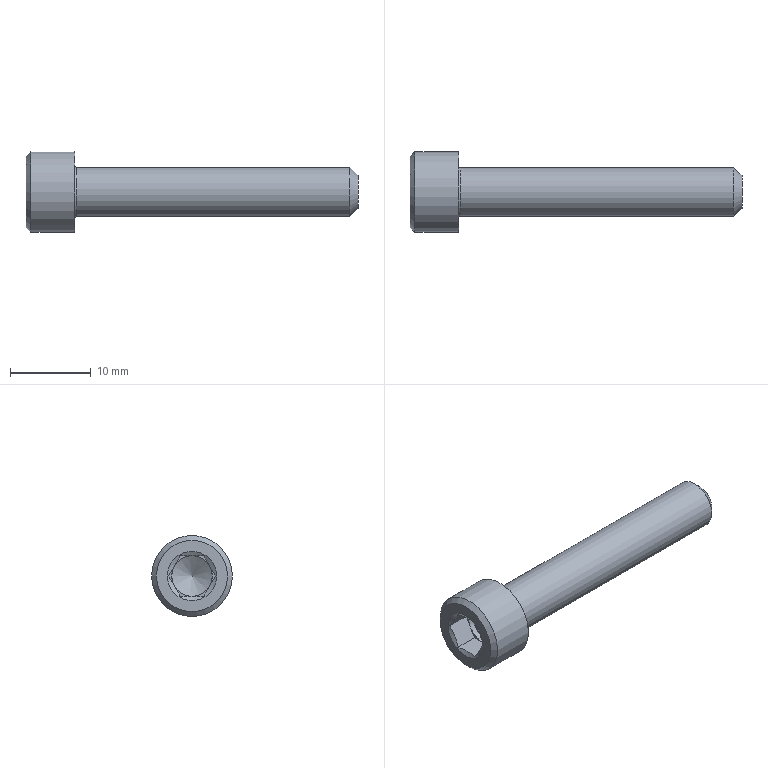Part | STEP file | Винт М6-6gx35 ГОСТ 11738-84 | 1 solid | 23 faces | box 41 x 10 x 10 mm | volume 1358 mm3 | plane 15 | cone 4 | cylinder 3 | torus 1 | commonest cylinder face diameters 5 x1 6 x1 10 x1
STEP:
#1=CARTESIAN_POINT('',(-6.,4.4,0.));
#2=VERTEX_POINT('',#1);
#3=CARTESIAN_POINT('',(-6.,0.,0.));
#4=DIRECTION('',(1.,0.,0.));
#5=DIRECTION('',(0.,1.,0.));
#6=AXIS2_PLACEMENT_3D('',#3,#4,#5);
#7=CIRCLE('',#6,4.4);
#8=EDGE_CURVE('',#2,#2,#7,.T.);
#9=ORIENTED_EDGE('',*,*,#8,.F.);
#10=EDGE_LOOP('',(#9));
#11=FACE_BOUND('',#10,.T.);
#12=CARTESIAN_POINT('',(-6.,3.05,0.));
#13=VERTEX_POINT('',#12);
#14=CARTESIAN_POINT('',(-6.,0.,0.));
#15=DIRECTION('',(1.,0.,0.));
#16=DIRECTION('',(0.,1.,0.));
#17=AXIS2_PLACEMENT_3D('',#14,#15,#16);
#18=CIRCLE('',#17,3.05);
#19=EDGE_CURVE('',#13,#13,#18,.T.);
#20=ORIENTED_EDGE('',*,*,#19,.T.);
#21=EDGE_LOOP('',(#20));
#22=FACE_BOUND('',#21,.T.);
#23=CARTESIAN_POINT('',(-6.,0.,0.));
#24=DIRECTION('',(-1.,0.,0.));
#25=DIRECTION('',(0.,1.,0.));
#26=AXIS2_PLACEMENT_3D('',#23,#24,#25);
#27=PLANE('',#26);
#28=ADVANCED_FACE('',(#11,#22),#27,.T.);
#29=CARTESIAN_POINT('',(-5.906,1.443,-2.5));
#30=VERTEX_POINT('',#29);
#31=CARTESIAN_POINT('',(-5.906,-1.443,-2.5));
#32=VERTEX_POINT('',#31);
#33=CARTESIAN_POINT('',(-5.906,1.443,-2.5));
#34=CARTESIAN_POINT('',(-5.9,1.424,-2.5));
#35=CARTESIAN_POINT('',(-5.89,1.389,-2.5));
#36=CARTESIAN_POINT('',(-5.88,1.351,-2.5));
#37=CARTESIAN_POINT('',(-5.867,1.304,-2.5));
#38=CARTESIAN_POINT('',(-5.848,1.232,-2.5));
#39=CARTESIAN_POINT('',(-5.827,1.146,-2.5));
#40=CARTESIAN_POINT('',(-5.803,1.043,-2.5));
#41=CARTESIAN_POINT('',(-5.774,0.909,-2.5));
#42=CARTESIAN_POINT('',(-5.75,0.7773,-2.5));
#43=CARTESIAN_POINT('',(-5.728,0.6356,-2.5));
#44=CARTESIAN_POINT('',(-5.711,0.5115,-2.5));
#45=CARTESIAN_POINT('',(-5.699,0.3892,-2.5));
#46=CARTESIAN_POINT('',(-5.692,0.2947,-2.5));
#47=CARTESIAN_POINT('',(-5.688,0.2222,-2.5));
#48=CARTESIAN_POINT('',(-5.684,0.1323,-2.5));
#49=CARTESIAN_POINT('',(-5.683,0.05578,-2.5));
#50=CARTESIAN_POINT('',(-5.682,-0.001577,-2.5));
#51=CARTESIAN_POINT('',(-5.683,-0.03169,-2.5));
#52=CARTESIAN_POINT('',(-5.683,-0.0738,-2.5));
#53=CARTESIAN_POINT('',(-5.684,-0.1276,-2.5));
#54=CARTESIAN_POINT('',(-5.687,-0.2055,-2.5));
#55=CARTESIAN_POINT('',(-5.692,-0.2839,-2.5));
#56=CARTESIAN_POINT('',(-5.696,-0.3444,-2.5));
#57=CARTESIAN_POINT('',(-5.7,-0.3959,-2.5));
#58=CARTESIAN_POINT('',(-5.705,-0.4472,-2.5));
#59=CARTESIAN_POINT('',(-5.713,-0.5148,-2.5));
#60=CARTESIAN_POINT('',(-5.722,-0.5907,-2.5));
#61=CARTESIAN_POINT('',(-5.73,-0.6507,-2.5));
#62=CARTESIAN_POINT('',(-5.738,-0.7005,-2.5));
#63=CARTESIAN_POINT('',(-5.746,-0.7498,-2.5));
#64=CARTESIAN_POINT('',(-5.757,-0.8136,-2.5));
#65=CARTESIAN_POINT('',(-5.77,-0.8864,-2.5));
#66=CARTESIAN_POINT('',(-5.785,-0.9583,-2.5));
#67=CARTESIAN_POINT('',(-5.8,-1.03,-2.5));
#68=CARTESIAN_POINT('',(-5.812,-1.084,-2.5));
#69=CARTESIAN_POINT('',(-5.823,-1.131,-2.5));
#70=CARTESIAN_POINT('',(-5.834,-1.177,-2.5));
#71=CARTESIAN_POINT('',(-5.85,-1.239,-2.5));
#72=CARTESIAN_POINT('',(-5.868,-1.307,-2.5));
#73=CARTESIAN_POINT('',(-5.882,-1.361,-2.5));
#74=CARTESIAN_POINT('',(-5.895,-1.406,-2.5));
#75=CARTESIAN_POINT('',(-5.902,-1.429,-2.5));
#76=CARTESIAN_POINT('',(-5.906,-1.443,-2.5));
#77=B_SPLINE_CURVE_WITH_KNOTS('',3,(#33,#34,#35,#36,#37,#38,#39,#40,#41,#42,#43,#44,#45,#46,#47,#48,#49,#50,#51,#52,#53,#54,#55,#56,#57,#58,#59,#60,#61,#62,#63,#64,#65,#66,#67,#68,#69,#70,#71,#72,#73,#74,#75,#76),.UNSPECIFIED.,.F.,.F.,(4,1,1,1,1,1,1,1,1,1,1,1,1,1,1,1,1,1,1,1,1,1,1,1,1,1,1,1,1,1,1,1,1,1,1,1,1,1,1,1,1,4),(0.,0.02097,0.03685,0.04095,0.07015,0.1134,0.1316,0.1778,0.2541,0.2686,0.3246,0.3823,0.3943,0.4217,0.4566,0.4863,0.5,0.5153,0.5171,0.5431,0.5703,0.5969,0.6234,0.6325,0.6498,0.6761,0.7022,0.7281,0.7381,0.7538,0.7792,0.8044,0.8294,0.8543,0.8789,0.8866,0.9033,0.9276,0.9518,0.9759,0.9843,1.),.UNSPECIFIED.);
#78=EDGE_CURVE('',#30,#32,#77,.T.);
#79=ORIENTED_EDGE('',*,*,#78,.T.);
#80=CARTESIAN_POINT('',(-3.,-1.443,-2.5));
#81=VERTEX_POINT('',#80);
#82=CARTESIAN_POINT('',(-3.,-1.443,-2.5));
#83=DIRECTION('',(-1.,0.,0.));
#84=VECTOR('',#83,1.);
#85=LINE('',#82,#84);
#86=EDGE_CURVE('',#81,#32,#85,.T.);
#87=ORIENTED_EDGE('',*,*,#86,.F.);
#88=CARTESIAN_POINT('',(-3.,0.,-2.5));
#89=VERTEX_POINT('',#88);
#90=CARTESIAN_POINT('',(-3.,0.,-2.5));
#91=DIRECTION('',(0.,-1.,0.));
#92=VECTOR('',#91,1.);
#93=LINE('',#90,#92);
#94=EDGE_CURVE('',#89,#81,#93,.T.);
#95=ORIENTED_EDGE('',*,*,#94,.F.);
#96=CARTESIAN_POINT('',(-3.,1.443,-2.5));
#97=VERTEX_POINT('',#96);
#98=CARTESIAN_POINT('',(-3.,1.443,-2.5));
#99=DIRECTION('',(0.,-1.,0.));
#100=VECTOR('',#99,1.);
#101=LINE('',#98,#100);
#102=EDGE_CURVE('',#97,#89,#101,.T.);
#103=ORIENTED_EDGE('',*,*,#102,.F.);
#104=CARTESIAN_POINT('',(-3.,1.443,-2.5));
#105=DIRECTION('',(-1.,0.,0.));
#106=VECTOR('',#105,1.);
#107=LINE('',#104,#106);
#108=EDGE_CURVE('',#97,#30,#107,.T.);
#109=ORIENTED_EDGE('',*,*,#108,.T.);
#110=EDGE_LOOP('',(#79,#87,#95,#103,#109));
#111=FACE_BOUND('',#110,.T.);
#112=CARTESIAN_POINT('',(-3.,1.443,-2.5));
#113=DIRECTION('',(0.,0.,-1.));
#114=DIRECTION('',(0.,-1.,0.));
#115=AXIS2_PLACEMENT_3D('',#112,#113,#114);
#116=PLANE('',#115);
#117=ADVANCED_FACE('',(#111),#116,.F.);
#118=CARTESIAN_POINT('',(-5.906,-2.887,0.));
#119=VERTEX_POINT('',#118);
#120=CARTESIAN_POINT('',(-5.906,-1.443,-2.5));
#121=CARTESIAN_POINT('',(-5.9,-1.453,-2.483));
#122=CARTESIAN_POINT('',(-5.889,-1.472,-2.45));
#123=CARTESIAN_POINT('',(-5.871,-1.505,-2.392));
#124=CARTESIAN_POINT('',(-5.848,-1.549,-2.317));
#125=CARTESIAN_POINT('',(-5.816,-1.614,-2.204));
#126=CARTESIAN_POINT('',(-5.777,-1.702,-2.052));
#127=CARTESIAN_POINT('',(-5.74,-1.803,-1.877));
#128=CARTESIAN_POINT('',(-5.713,-1.902,-1.705));
#129=CARTESIAN_POINT('',(-5.697,-1.984,-1.564));
#130=CARTESIAN_POINT('',(-5.688,-2.048,-1.453));
#131=CARTESIAN_POINT('',(-5.684,-2.099,-1.365));
#132=CARTESIAN_POINT('',(-5.683,-2.137,-1.298));
#133=CARTESIAN_POINT('',(-5.682,-2.166,-1.249));
#134=CARTESIAN_POINT('',(-5.683,-2.194,-1.201));
#135=CARTESIAN_POINT('',(-5.684,-2.228,-1.141));
#136=CARTESIAN_POINT('',(-5.687,-2.268,-1.072));
#137=CARTESIAN_POINT('',(-5.692,-2.307,-1.004));
#138=CARTESIAN_POINT('',(-5.697,-2.346,-0.9371));
#139=CARTESIAN_POINT('',(-5.704,-2.384,-0.8704));
#140=CARTESIAN_POINT('',(-5.713,-2.422,-0.8041));
#141=CARTESIAN_POINT('',(-5.722,-2.46,-0.7384));
#142=CARTESIAN_POINT('',(-5.733,-2.498,-0.6734));
#143=CARTESIAN_POINT('',(-5.744,-2.535,-0.609));
#144=CARTESIAN_POINT('',(-5.757,-2.572,-0.5454));
#145=CARTESIAN_POINT('',(-5.77,-2.608,-0.4824));
#146=CARTESIAN_POINT('',(-5.785,-2.644,-0.4201));
#147=CARTESIAN_POINT('',(-5.8,-2.68,-0.3584));
#148=CARTESIAN_POINT('',(-5.816,-2.715,-0.2974));
#149=CARTESIAN_POINT('',(-5.832,-2.75,-0.237));
#150=CARTESIAN_POINT('',(-5.85,-2.784,-0.1771));
#151=CARTESIAN_POINT('',(-5.868,-2.819,-0.1177));
#152=CARTESIAN_POINT('',(-5.886,-2.853,-0.05869));
#153=CARTESIAN_POINT('',(-5.899,-2.875,-0.01952));
#154=CARTESIAN_POINT('',(-5.906,-2.887,0.));
#155=B_SPLINE_CURVE_WITH_KNOTS('',3,(#120,#121,#122,#123,#124,#125,#126,#127,#128,#129,#130,#131,#132,#133,#134,#135,#136,#137,#138,#139,#140,#141,#142,#143,#144,#145,#146,#147,#148,#149,#150,#151,#152,#153,#154),.UNSPECIFIED.,.F.,.F.,(4,1,1,1,1,1,1,1,1,1,1,1,1,1,1,1,1,1,1,1,1,1,1,1,1,1,1,1,1,1,1,1,4),(0.,0.02097,0.04095,0.07015,0.1134,0.1778,0.2541,0.3246,0.3823,0.4217,0.4566,0.4863,0.5,0.5153,0.5431,0.5703,0.5969,0.6234,0.6498,0.6761,0.7022,0.7281,0.7538,0.7792,0.8044,0.8294,0.8543,0.8789,0.9033,0.9276,0.9518,0.9759,1.),.UNSPECIFIED.);
#156=EDGE_CURVE('',#32,#119,#155,.T.);
#157=ORIENTED_EDGE('',*,*,#156,.T.);
#158=CARTESIAN_POINT('',(-3.,-2.887,0.));
#159=VERTEX_POINT('',#158);
#160=CARTESIAN_POINT('',(-3.,-2.887,0.));
#161=DIRECTION('',(-1.,0.,0.));
#162=VECTOR('',#161,1.);
#163=LINE('',#160,#162);
#164=EDGE_CURVE('',#159,#119,#163,.T.);
#165=ORIENTED_EDGE('',*,*,#164,.F.);
#166=CARTESIAN_POINT('',(-3.,-2.165,-1.25));
#167=VERTEX_POINT('',#166);
#168=CARTESIAN_POINT('',(-3.,-2.165,-1.25));
#169=DIRECTION('',(0.,-0.5,0.866));
#170=VECTOR('',#169,1.);
#171=LINE('',#168,#170);
#172=EDGE_CURVE('',#167,#159,#171,.T.);
#173=ORIENTED_EDGE('',*,*,#172,.F.);
#174=CARTESIAN_POINT('',(-3.,-1.443,-2.5));
#175=DIRECTION('',(0.,-0.5,0.866));
#176=VECTOR('',#175,1.);
#177=LINE('',#174,#176);
#178=EDGE_CURVE('',#81,#167,#177,.T.);
#179=ORIENTED_EDGE('',*,*,#178,.F.);
#180=ORIENTED_EDGE('',*,*,#86,.T.);
#181=EDGE_LOOP('',(#157,#165,#173,#179,#180));
#182=FACE_BOUND('',#181,.T.);
#183=CARTESIAN_POINT('',(-3.,-1.443,-2.5));
#184=DIRECTION('',(0.,-0.866,-0.5));
#185=DIRECTION('',(0.,-0.5,0.866));
#186=AXIS2_PLACEMENT_3D('',#183,#184,#185);
#187=PLANE('',#186);
#188=ADVANCED_FACE('',(#182),#187,.F.);
#189=CARTESIAN_POINT('',(-5.906,-1.443,2.5));
#190=VERTEX_POINT('',#189);
#191=CARTESIAN_POINT('',(-5.906,-2.887,0.));
#192=CARTESIAN_POINT('',(-5.9,-2.877,0.01704));
#193=CARTESIAN_POINT('',(-5.889,-2.858,0.05036));
#194=CARTESIAN_POINT('',(-5.871,-2.825,0.1076));
#195=CARTESIAN_POINT('',(-5.848,-2.781,0.1832));
#196=CARTESIAN_POINT('',(-5.816,-2.716,0.2956));
#197=CARTESIAN_POINT('',(-5.777,-2.628,0.4476));
#198=CARTESIAN_POINT('',(-5.74,-2.527,0.6235));
#199=CARTESIAN_POINT('',(-5.713,-2.428,0.7948));
#200=CARTESIAN_POINT('',(-5.697,-2.346,0.936));
#201=CARTESIAN_POINT('',(-5.688,-2.282,1.047));
#202=CARTESIAN_POINT('',(-5.684,-2.231,1.135));
#203=CARTESIAN_POINT('',(-5.683,-2.193,1.202));
#204=CARTESIAN_POINT('',(-5.682,-2.164,1.251));
#205=CARTESIAN_POINT('',(-5.683,-2.137,1.299));
#206=CARTESIAN_POINT('',(-5.684,-2.102,1.359));
#207=CARTESIAN_POINT('',(-5.687,-2.062,1.428));
#208=CARTESIAN_POINT('',(-5.692,-2.023,1.496));
#209=CARTESIAN_POINT('',(-5.697,-1.984,1.563));
#210=CARTESIAN_POINT('',(-5.704,-1.946,1.63));
#211=CARTESIAN_POINT('',(-5.713,-1.908,1.696));
#212=CARTESIAN_POINT('',(-5.722,-1.87,1.762));
#213=CARTESIAN_POINT('',(-5.733,-1.832,1.827));
#214=CARTESIAN_POINT('',(-5.744,-1.795,1.891));
#215=CARTESIAN_POINT('',(-5.757,-1.758,1.955));
#216=CARTESIAN_POINT('',(-5.77,-1.722,2.018));
#217=CARTESIAN_POINT('',(-5.785,-1.686,2.08));
#218=CARTESIAN_POINT('',(-5.8,-1.65,2.142));
#219=CARTESIAN_POINT('',(-5.816,-1.615,2.203));
#220=CARTESIAN_POINT('',(-5.832,-1.58,2.263));
#221=CARTESIAN_POINT('',(-5.85,-1.546,2.323));
#222=CARTESIAN_POINT('',(-5.868,-1.511,2.382));
#223=CARTESIAN_POINT('',(-5.886,-1.477,2.441));
#224=CARTESIAN_POINT('',(-5.899,-1.455,2.48));
#225=CARTESIAN_POINT('',(-5.906,-1.443,2.5));
#226=B_SPLINE_CURVE_WITH_KNOTS('',3,(#191,#192,#193,#194,#195,#196,#197,#198,#199,#200,#201,#202,#203,#204,#205,#206,#207,#208,#209,#210,#211,#212,#213,#214,#215,#216,#217,#218,#219,#220,#221,#222,#223,#224,#225),.UNSPECIFIED.,.F.,.F.,(4,1,1,1,1,1,1,1,1,1,1,1,1,1,1,1,1,1,1,1,1,1,1,1,1,1,1,1,1,1,1,1,4),(0.,0.02097,0.04095,0.07015,0.1134,0.1778,0.2541,0.3246,0.3823,0.4217,0.4566,0.4863,0.5,0.5153,0.5431,0.5703,0.5969,0.6234,0.6498,0.6761,0.7022,0.7281,0.7538,0.7792,0.8044,0.8294,0.8543,0.8789,0.9033,0.9276,0.9518,0.9759,1.),.UNSPECIFIED.);
#227=EDGE_CURVE('',#119,#190,#226,.T.);
#228=ORIENTED_EDGE('',*,*,#227,.T.);
#229=CARTESIAN_POINT('',(-3.,-1.443,2.5));
#230=VERTEX_POINT('',#229);
#231=CARTESIAN_POINT('',(-3.,-1.443,2.5));
#232=DIRECTION('',(-1.,0.,0.));
#233=VECTOR('',#232,1.);
#234=LINE('',#231,#233);
#235=EDGE_CURVE('',#230,#190,#234,.T.);
#236=ORIENTED_EDGE('',*,*,#235,.F.);
#237=CARTESIAN_POINT('',(-3.,-2.165,1.25));
#238=VERTEX_POINT('',#237);
#239=CARTESIAN_POINT('',(-3.,-2.165,1.25));
#240=DIRECTION('',(0.,0.5,0.866));
#241=VECTOR('',#240,1.);
#242=LINE('',#239,#241);
#243=EDGE_CURVE('',#238,#230,#242,.T.);
#244=ORIENTED_EDGE('',*,*,#243,.F.);
#245=CARTESIAN_POINT('',(-3.,-2.887,0.));
#246=DIRECTION('',(0.,0.5,0.866));
#247=VECTOR('',#246,1.);
#248=LINE('',#245,#247);
#249=EDGE_CURVE('',#159,#238,#248,.T.);
#250=ORIENTED_EDGE('',*,*,#249,.F.);
#251=ORIENTED_EDGE('',*,*,#164,.T.);
#252=EDGE_LOOP('',(#228,#236,#244,#250,#251));
#253=FACE_BOUND('',#252,.T.);
#254=CARTESIAN_POINT('',(-3.,-2.887,0.));
#255=DIRECTION('',(0.,-0.866,0.5));
#256=DIRECTION('',(0.,0.5,0.866));
#257=AXIS2_PLACEMENT_3D('',#254,#255,#256);
#258=PLANE('',#257);
#259=ADVANCED_FACE('',(#253),#258,.F.);
#260=CARTESIAN_POINT('',(-5.906,1.443,2.5));
#261=VERTEX_POINT('',#260);
#262=CARTESIAN_POINT('',(-5.906,-1.443,2.5));
#263=CARTESIAN_POINT('',(-5.9,-1.424,2.5));
#264=CARTESIAN_POINT('',(-5.89,-1.389,2.5));
#265=CARTESIAN_POINT('',(-5.88,-1.351,2.5));
#266=CARTESIAN_POINT('',(-5.867,-1.304,2.5));
#267=CARTESIAN_POINT('',(-5.848,-1.232,2.5));
#268=CARTESIAN_POINT('',(-5.827,-1.146,2.5));
#269=CARTESIAN_POINT('',(-5.803,-1.043,2.5));
#270=CARTESIAN_POINT('',(-5.774,-0.909,2.5));
#271=CARTESIAN_POINT('',(-5.75,-0.7773,2.5));
#272=CARTESIAN_POINT('',(-5.728,-0.6356,2.5));
#273=CARTESIAN_POINT('',(-5.711,-0.5115,2.5));
#274=CARTESIAN_POINT('',(-5.699,-0.3892,2.5));
#275=CARTESIAN_POINT('',(-5.692,-0.2947,2.5));
#276=CARTESIAN_POINT('',(-5.688,-0.2222,2.5));
#277=CARTESIAN_POINT('',(-5.684,-0.1323,2.5));
#278=CARTESIAN_POINT('',(-5.683,-0.05578,2.5));
#279=CARTESIAN_POINT('',(-5.682,0.001577,2.5));
#280=CARTESIAN_POINT('',(-5.683,0.03169,2.5));
#281=CARTESIAN_POINT('',(-5.683,0.0738,2.5));
#282=CARTESIAN_POINT('',(-5.684,0.1276,2.5));
#283=CARTESIAN_POINT('',(-5.687,0.2055,2.5));
#284=CARTESIAN_POINT('',(-5.692,0.2839,2.5));
#285=CARTESIAN_POINT('',(-5.696,0.3444,2.5));
#286=CARTESIAN_POINT('',(-5.7,0.3959,2.5));
#287=CARTESIAN_POINT('',(-5.705,0.4472,2.5));
#288=CARTESIAN_POINT('',(-5.713,0.5148,2.5));
#289=CARTESIAN_POINT('',(-5.722,0.5907,2.5));
#290=CARTESIAN_POINT('',(-5.73,0.6507,2.5));
#291=CARTESIAN_POINT('',(-5.738,0.7005,2.5));
#292=CARTESIAN_POINT('',(-5.746,0.7498,2.5));
#293=CARTESIAN_POINT('',(-5.757,0.8136,2.5));
#294=CARTESIAN_POINT('',(-5.77,0.8864,2.5));
#295=CARTESIAN_POINT('',(-5.785,0.9583,2.5));
#296=CARTESIAN_POINT('',(-5.8,1.03,2.5));
#297=CARTESIAN_POINT('',(-5.812,1.084,2.5));
#298=CARTESIAN_POINT('',(-5.823,1.131,2.5));
#299=CARTESIAN_POINT('',(-5.834,1.177,2.5));
#300=CARTESIAN_POINT('',(-5.85,1.239,2.5));
#301=CARTESIAN_POINT('',(-5.868,1.307,2.5));
#302=CARTESIAN_POINT('',(-5.882,1.361,2.5));
#303=CARTESIAN_POINT('',(-5.895,1.406,2.5));
#304=CARTESIAN_POINT('',(-5.902,1.429,2.5));
#305=CARTESIAN_POINT('',(-5.906,1.443,2.5));
#306=B_SPLINE_CURVE_WITH_KNOTS('',3,(#262,#263,#264,#265,#266,#267,#268,#269,#270,#271,#272,#273,#274,#275,#276,#277,#278,#279,#280,#281,#282,#283,#284,#285,#286,#287,#288,#289,#290,#291,#292,#293,#294,#295,#296,#297,#298,#299,#300,#301,#302,#303,#304,#305),.UNSPECIFIED.,.F.,.F.,(4,1,1,1,1,1,1,1,1,1,1,1,1,1,1,1,1,1,1,1,1,1,1,1,1,1,1,1,1,1,1,1,1,1,1,1,1,1,1,1,1,4),(0.,0.02097,0.03685,0.04095,0.07015,0.1134,0.1316,0.1778,0.2541,0.2686,0.3246,0.3823,0.3943,0.4217,0.4566,0.4863,0.5,0.5153,0.5171,0.5431,0.5703,0.5969,0.6234,0.6325,0.6498,0.6761,0.7022,0.7281,0.7381,0.7538,0.7792,0.8044,0.8294,0.8543,0.8789,0.8866,0.9033,0.9276,0.9518,0.9759,0.9843,1.),.UNSPECIFIED.);
#307=EDGE_CURVE('',#190,#261,#306,.T.);
#308=ORIENTED_EDGE('',*,*,#307,.T.);
#309=CARTESIAN_POINT('',(-3.,1.443,2.5));
#310=VERTEX_POINT('',#309);
#311=CARTESIAN_POINT('',(-3.,1.443,2.5));
#312=DIRECTION('',(-1.,0.,0.));
#313=VECTOR('',#312,1.);
#314=LINE('',#311,#313);
#315=EDGE_CURVE('',#310,#261,#314,.T.);
#316=ORIENTED_EDGE('',*,*,#315,.F.);
#317=CARTESIAN_POINT('',(-3.,0.,2.5));
#318=VERTEX_POINT('',#317);
#319=CARTESIAN_POINT('',(-3.,0.,2.5));
#320=DIRECTION('',(0.,1.,0.));
#321=VECTOR('',#320,1.);
#322=LINE('',#319,#321);
#323=EDGE_CURVE('',#318,#310,#322,.T.);
#324=ORIENTED_EDGE('',*,*,#323,.F.);
#325=CARTESIAN_POINT('',(-3.,-1.443,2.5));
#326=DIRECTION('',(0.,1.,0.));
#327=VECTOR('',#326,1.);
#328=LINE('',#325,#327);
#329=EDGE_CURVE('',#230,#318,#328,.T.);
#330=ORIENTED_EDGE('',*,*,#329,.F.);
#331=ORIENTED_EDGE('',*,*,#235,.T.);
#332=EDGE_LOOP('',(#308,#316,#324,#330,#331));
#333=FACE_BOUND('',#332,.T.);
#334=CARTESIAN_POINT('',(-3.,-1.443,2.5));
#335=DIRECTION('',(0.,0.,1.));
#336=DIRECTION('',(0.,1.,0.));
#337=AXIS2_PLACEMENT_3D('',#334,#335,#336);
#338=PLANE('',#337);
#339=ADVANCED_FACE('',(#333),#338,.F.);
#340=CARTESIAN_POINT('',(-5.906,2.887,0.));
#341=VERTEX_POINT('',#340);
#342=CARTESIAN_POINT('',(-5.906,2.887,0.));
#343=CARTESIAN_POINT('',(-5.9,2.877,-0.01704));
#344=CARTESIAN_POINT('',(-5.889,2.858,-0.05036));
#345=CARTESIAN_POINT('',(-5.871,2.825,-0.1076));
#346=CARTESIAN_POINT('',(-5.848,2.781,-0.1832));
#347=CARTESIAN_POINT('',(-5.816,2.716,-0.2956));
#348=CARTESIAN_POINT('',(-5.777,2.628,-0.4476));
#349=CARTESIAN_POINT('',(-5.74,2.527,-0.6235));
#350=CARTESIAN_POINT('',(-5.713,2.428,-0.7948));
#351=CARTESIAN_POINT('',(-5.697,2.346,-0.936));
#352=CARTESIAN_POINT('',(-5.688,2.282,-1.047));
#353=CARTESIAN_POINT('',(-5.684,2.231,-1.135));
#354=CARTESIAN_POINT('',(-5.683,2.193,-1.202));
#355=CARTESIAN_POINT('',(-5.682,2.164,-1.251));
#356=CARTESIAN_POINT('',(-5.683,2.137,-1.299));
#357=CARTESIAN_POINT('',(-5.684,2.102,-1.359));
#358=CARTESIAN_POINT('',(-5.687,2.062,-1.428));
#359=CARTESIAN_POINT('',(-5.692,2.023,-1.496));
#360=CARTESIAN_POINT('',(-5.697,1.984,-1.563));
#361=CARTESIAN_POINT('',(-5.704,1.946,-1.63));
#362=CARTESIAN_POINT('',(-5.713,1.908,-1.696));
#363=CARTESIAN_POINT('',(-5.722,1.87,-1.762));
#364=CARTESIAN_POINT('',(-5.733,1.832,-1.827));
#365=CARTESIAN_POINT('',(-5.744,1.795,-1.891));
#366=CARTESIAN_POINT('',(-5.757,1.758,-1.955));
#367=CARTESIAN_POINT('',(-5.77,1.722,-2.018));
#368=CARTESIAN_POINT('',(-5.785,1.686,-2.08));
#369=CARTESIAN_POINT('',(-5.8,1.65,-2.142));
#370=CARTESIAN_POINT('',(-5.816,1.615,-2.203));
#371=CARTESIAN_POINT('',(-5.832,1.58,-2.263));
#372=CARTESIAN_POINT('',(-5.85,1.546,-2.323));
#373=CARTESIAN_POINT('',(-5.868,1.511,-2.382));
#374=CARTESIAN_POINT('',(-5.886,1.477,-2.441));
#375=CARTESIAN_POINT('',(-5.899,1.455,-2.48));
#376=CARTESIAN_POINT('',(-5.906,1.443,-2.5));
#377=B_SPLINE_CURVE_WITH_KNOTS('',3,(#342,#343,#344,#345,#346,#347,#348,#349,#350,#351,#352,#353,#354,#355,#356,#357,#358,#359,#360,#361,#362,#363,#364,#365,#366,#367,#368,#369,#370,#371,#372,#373,#374,#375,#376),.UNSPECIFIED.,.F.,.F.,(4,1,1,1,1,1,1,1,1,1,1,1,1,1,1,1,1,1,1,1,1,1,1,1,1,1,1,1,1,1,1,1,4),(0.,0.02097,0.04095,0.07015,0.1134,0.1778,0.2541,0.3246,0.3823,0.4217,0.4566,0.4863,0.5,0.5153,0.5431,0.5703,0.5969,0.6234,0.6498,0.6761,0.7022,0.7281,0.7538,0.7792,0.8044,0.8294,0.8543,0.8789,0.9033,0.9276,0.9518,0.9759,1.),.UNSPECIFIED.);
#378=EDGE_CURVE('',#341,#30,#377,.T.);
#379=ORIENTED_EDGE('',*,*,#378,.T.);
#380=ORIENTED_EDGE('',*,*,#108,.F.);
#381=CARTESIAN_POINT('',(-3.,2.165,-1.25));
#382=VERTEX_POINT('',#381);
#383=CARTESIAN_POINT('',(-3.,2.165,-1.25));
#384=DIRECTION('',(0.,-0.5,-0.866));
#385=VECTOR('',#384,1.);
#386=LINE('',#383,#385);
#387=EDGE_CURVE('',#382,#97,#386,.T.);
#388=ORIENTED_EDGE('',*,*,#387,.F.);
#389=CARTESIAN_POINT('',(-3.,2.887,0.));
#390=VERTEX_POINT('',#389);
#391=CARTESIAN_POINT('',(-3.,2.887,0.));
#392=DIRECTION('',(0.,-0.5,-0.866));
#393=VECTOR('',#392,1.);
#394=LINE('',#391,#393);
#395=EDGE_CURVE('',#390,#382,#394,.T.);
#396=ORIENTED_EDGE('',*,*,#395,.F.);
#397=CARTESIAN_POINT('',(-3.,2.887,0.));
#398=DIRECTION('',(-1.,0.,0.));
#399=VECTOR('',#398,1.);
#400=LINE('',#397,#399);
#401=EDGE_CURVE('',#390,#341,#400,.T.);
#402=ORIENTED_EDGE('',*,*,#401,.T.);
#403=EDGE_LOOP('',(#379,#380,#388,#396,#402));
#404=FACE_BOUND('',#403,.T.);
#405=CARTESIAN_POINT('',(-3.,2.887,0.));
#406=DIRECTION('',(0.,0.866,-0.5));
#407=DIRECTION('',(0.,-0.5,-0.866));
#408=AXIS2_PLACEMENT_3D('',#405,#406,#407);
#409=PLANE('',#408);
#410=ADVANCED_FACE('',(#404),#409,.F.);
#411=CARTESIAN_POINT('',(-5.906,1.443,2.5));
#412=CARTESIAN_POINT('',(-5.9,1.453,2.483));
#413=CARTESIAN_POINT('',(-5.889,1.472,2.45));
#414=CARTESIAN_POINT('',(-5.871,1.505,2.392));
#415=CARTESIAN_POINT('',(-5.848,1.549,2.317));
#416=CARTESIAN_POINT('',(-5.816,1.614,2.204));
#417=CARTESIAN_POINT('',(-5.777,1.702,2.052));
#418=CARTESIAN_POINT('',(-5.74,1.803,1.877));
#419=CARTESIAN_POINT('',(-5.713,1.902,1.705));
#420=CARTESIAN_POINT('',(-5.697,1.984,1.564));
#421=CARTESIAN_POINT('',(-5.688,2.048,1.453));
#422=CARTESIAN_POINT('',(-5.684,2.099,1.365));
#423=CARTESIAN_POINT('',(-5.683,2.137,1.298));
#424=CARTESIAN_POINT('',(-5.682,2.166,1.249));
#425=CARTESIAN_POINT('',(-5.683,2.194,1.201));
#426=CARTESIAN_POINT('',(-5.684,2.228,1.141));
#427=CARTESIAN_POINT('',(-5.687,2.268,1.072));
#428=CARTESIAN_POINT('',(-5.692,2.307,1.004));
#429=CARTESIAN_POINT('',(-5.697,2.346,0.9371));
#430=CARTESIAN_POINT('',(-5.704,2.384,0.8704));
#431=CARTESIAN_POINT('',(-5.713,2.422,0.8041));
#432=CARTESIAN_POINT('',(-5.722,2.46,0.7384));
#433=CARTESIAN_POINT('',(-5.733,2.498,0.6734));
#434=CARTESIAN_POINT('',(-5.744,2.535,0.609));
#435=CARTESIAN_POINT('',(-5.757,2.572,0.5454));
#436=CARTESIAN_POINT('',(-5.77,2.608,0.4824));
#437=CARTESIAN_POINT('',(-5.785,2.644,0.4201));
#438=CARTESIAN_POINT('',(-5.8,2.68,0.3584));
#439=CARTESIAN_POINT('',(-5.816,2.715,0.2974));
#440=CARTESIAN_POINT('',(-5.832,2.75,0.237));
#441=CARTESIAN_POINT('',(-5.85,2.784,0.1771));
#442=CARTESIAN_POINT('',(-5.868,2.819,0.1177));
#443=CARTESIAN_POINT('',(-5.886,2.853,0.05869));
#444=CARTESIAN_POINT('',(-5.899,2.875,0.01952));
#445=CARTESIAN_POINT('',(-5.906,2.887,0.));
#446=B_SPLINE_CURVE_WITH_KNOTS('',3,(#411,#412,#413,#414,#415,#416,#417,#418,#419,#420,#421,#422,#423,#424,#425,#426,#427,#428,#429,#430,#431,#432,#433,#434,#435,#436,#437,#438,#439,#440,#441,#442,#443,#444,#445),.UNSPECIFIED.,.F.,.F.,(4,1,1,1,1,1,1,1,1,1,1,1,1,1,1,1,1,1,1,1,1,1,1,1,1,1,1,1,1,1,1,1,4),(0.,0.02097,0.04095,0.07015,0.1134,0.1778,0.2541,0.3246,0.3823,0.4217,0.4566,0.4863,0.5,0.5153,0.5431,0.5703,0.5969,0.6234,0.6498,0.6761,0.7022,0.7281,0.7538,0.7792,0.8044,0.8294,0.8543,0.8789,0.9033,0.9276,0.9518,0.9759,1.),.UNSPECIFIED.);
#447=EDGE_CURVE('',#261,#341,#446,.T.);
#448=ORIENTED_EDGE('',*,*,#447,.T.);
#449=ORIENTED_EDGE('',*,*,#401,.F.);
#450=CARTESIAN_POINT('',(-3.,2.165,1.25));
#451=VERTEX_POINT('',#450);
#452=CARTESIAN_POINT('',(-3.,2.165,1.25));
#453=DIRECTION('',(0.,0.5,-0.866));
#454=VECTOR('',#453,1.);
#455=LINE('',#452,#454);
#456=EDGE_CURVE('',#451,#390,#455,.T.);
#457=ORIENTED_EDGE('',*,*,#456,.F.);
#458=CARTESIAN_POINT('',(-3.,1.443,2.5));
#459=DIRECTION('',(0.,0.5,-0.866));
#460=VECTOR('',#459,1.);
#461=LINE('',#458,#460);
#462=EDGE_CURVE('',#310,#451,#461,.T.);
#463=ORIENTED_EDGE('',*,*,#462,.F.);
#464=ORIENTED_EDGE('',*,*,#315,.T.);
#465=EDGE_LOOP('',(#448,#449,#457,#463,#464));
#466=FACE_BOUND('',#465,.T.);
#467=CARTESIAN_POINT('',(-3.,1.443,2.5));
#468=DIRECTION('',(0.,0.866,0.5));
#469=DIRECTION('',(0.,0.5,-0.866));
#470=AXIS2_PLACEMENT_3D('',#467,#468,#469);
#471=PLANE('',#470);
#472=ADVANCED_FACE('',(#466),#471,.F.);
#473=ORIENTED_EDGE('',*,*,#447,.F.);
#474=ORIENTED_EDGE('',*,*,#307,.F.);
#475=ORIENTED_EDGE('',*,*,#227,.F.);
#476=ORIENTED_EDGE('',*,*,#156,.F.);
#477=ORIENTED_EDGE('',*,*,#78,.F.);
#478=ORIENTED_EDGE('',*,*,#378,.F.);
#479=EDGE_LOOP('',(#473,#474,#475,#476,#477,#478));
#480=FACE_BOUND('',#479,.T.);
#481=ORIENTED_EDGE('',*,*,#19,.F.);
#482=EDGE_LOOP('',(#481));
#483=FACE_OUTER_BOUND('',#482,.T.);
#484=CARTESIAN_POINT('',(-5.841,0.,0.));
#485=DIRECTION('',(-1.,0.,0.));
#486=DIRECTION('',(0.,-1.,0.));
#487=AXIS2_PLACEMENT_3D('',#484,#485,#486);
#488=CONICAL_SURFACE('',#487,2.775,1.047);
#489=ADVANCED_FACE('',(#480,#483),#488,.F.);
#490=CARTESIAN_POINT('',(-5.4,5.,0.));
#491=VERTEX_POINT('',#490);
#492=CARTESIAN_POINT('',(-5.4,0.,0.));
#493=DIRECTION('',(1.,0.,0.));
#494=DIRECTION('',(0.,1.,0.));
#495=AXIS2_PLACEMENT_3D('',#492,#493,#494);
#496=CIRCLE('',#495,5.);
#497=EDGE_CURVE('',#491,#491,#496,.T.);
#498=ORIENTED_EDGE('',*,*,#497,.F.);
#499=EDGE_LOOP('',(#498));
#500=FACE_OUTER_BOUND('',#499,.T.);
#501=ORIENTED_EDGE('',*,*,#8,.T.);
#502=EDGE_LOOP('',(#501));
#503=FACE_OUTER_BOUND('',#502,.T.);
#504=CARTESIAN_POINT('',(-5.7,0.,0.));
#505=DIRECTION('',(1.,0.,0.));
#506=DIRECTION('',(0.,1.,0.));
#507=AXIS2_PLACEMENT_3D('',#504,#505,#506);
#508=CONICAL_SURFACE('',#507,4.7,0.7854);
#509=ADVANCED_FACE('',(#500,#503),#508,.T.);
#510=CARTESIAN_POINT('',(-3.,0.,0.));
#511=DIRECTION('',(1.,0.,0.));
#512=DIRECTION('',(0.,-0.866,-0.5));
#513=AXIS2_PLACEMENT_3D('',#510,#511,#512);
#514=CIRCLE('',#513,2.5);
#515=EDGE_CURVE('',#167,#89,#514,.T.);
#516=ORIENTED_EDGE('',*,*,#515,.T.);
#517=ORIENTED_EDGE('',*,*,#94,.T.);
#518=ORIENTED_EDGE('',*,*,#178,.T.);
#519=EDGE_LOOP('',(#516,#517,#518));
#520=FACE_BOUND('',#519,.T.);
#521=CARTESIAN_POINT('',(-3.,0.,0.));
#522=DIRECTION('',(-1.,0.,0.));
#523=DIRECTION('',(0.,0.,-1.));
#524=AXIS2_PLACEMENT_3D('',#521,#522,#523);
#525=PLANE('',#524);
#526=ADVANCED_FACE('',(#520),#525,.T.);
#527=CARTESIAN_POINT('',(-3.,0.,0.));
#528=DIRECTION('',(1.,0.,0.));
#529=DIRECTION('',(0.,0.,-1.));
#530=AXIS2_PLACEMENT_3D('',#527,#528,#529);
#531=CIRCLE('',#530,2.5);
#532=EDGE_CURVE('',#89,#382,#531,.T.);
#533=ORIENTED_EDGE('',*,*,#532,.T.);
#534=ORIENTED_EDGE('',*,*,#387,.T.);
#535=ORIENTED_EDGE('',*,*,#102,.T.);
#536=EDGE_LOOP('',(#533,#534,#535));
#537=FACE_BOUND('',#536,.T.);
#538=CARTESIAN_POINT('',(-3.,0.,0.));
#539=DIRECTION('',(-1.,0.,0.));
#540=DIRECTION('',(0.,0.,-1.));
#541=AXIS2_PLACEMENT_3D('',#538,#539,#540);
#542=PLANE('',#541);
#543=ADVANCED_FACE('',(#537),#542,.T.);
#544=CARTESIAN_POINT('',(-3.,0.,0.));
#545=DIRECTION('',(1.,0.,0.));
#546=DIRECTION('',(0.,-0.866,0.5));
#547=AXIS2_PLACEMENT_3D('',#544,#545,#546);
#548=CIRCLE('',#547,2.5);
#549=EDGE_CURVE('',#238,#167,#548,.T.);
#550=ORIENTED_EDGE('',*,*,#549,.T.);
#551=ORIENTED_EDGE('',*,*,#172,.T.);
#552=ORIENTED_EDGE('',*,*,#249,.T.);
#553=EDGE_LOOP('',(#550,#551,#552));
#554=FACE_BOUND('',#553,.T.);
#555=CARTESIAN_POINT('',(-3.,0.,0.));
#556=DIRECTION('',(-1.,0.,0.));
#557=DIRECTION('',(0.,0.,-1.));
#558=AXIS2_PLACEMENT_3D('',#555,#556,#557);
#559=PLANE('',#558);
#560=ADVANCED_FACE('',(#554),#559,.T.);
#561=CARTESIAN_POINT('',(-3.,0.,0.));
#562=DIRECTION('',(1.,0.,0.));
#563=DIRECTION('',(0.,0.,1.));
#564=AXIS2_PLACEMENT_3D('',#561,#562,#563);
#565=CIRCLE('',#564,2.5);
#566=EDGE_CURVE('',#318,#238,#565,.T.);
#567=ORIENTED_EDGE('',*,*,#566,.T.);
#568=ORIENTED_EDGE('',*,*,#243,.T.);
#569=ORIENTED_EDGE('',*,*,#329,.T.);
#570=EDGE_LOOP('',(#567,#568,#569));
#571=FACE_BOUND('',#570,.T.);
#572=CARTESIAN_POINT('',(-3.,0.,0.));
#573=DIRECTION('',(-1.,0.,0.));
#574=DIRECTION('',(0.,0.,-1.));
#575=AXIS2_PLACEMENT_3D('',#572,#573,#574);
#576=PLANE('',#575);
#577=ADVANCED_FACE('',(#571),#576,.T.);
#578=CARTESIAN_POINT('',(-3.,0.,0.));
#579=DIRECTION('',(1.,0.,0.));
#580=DIRECTION('',(0.,0.866,0.5));
#581=AXIS2_PLACEMENT_3D('',#578,#579,#580);
#582=CIRCLE('',#581,2.5);
#583=EDGE_CURVE('',#451,#318,#582,.T.);
#584=ORIENTED_EDGE('',*,*,#583,.T.);
#585=ORIENTED_EDGE('',*,*,#323,.T.);
#586=ORIENTED_EDGE('',*,*,#462,.T.);
#587=EDGE_LOOP('',(#584,#585,#586));
#588=FACE_BOUND('',#587,.T.);
#589=CARTESIAN_POINT('',(-3.,0.,0.));
#590=DIRECTION('',(-1.,0.,0.));
#591=DIRECTION('',(0.,0.,-1.));
#592=AXIS2_PLACEMENT_3D('',#589,#590,#591);
#593=PLANE('',#592);
#594=ADVANCED_FACE('',(#588),#593,.T.);
#595=CARTESIAN_POINT('',(-3.,2.5,0.));
#596=VERTEX_POINT('',#595);
#597=CARTESIAN_POINT('',(-3.,0.,0.));
#598=DIRECTION('',(1.,0.,0.));
#599=DIRECTION('',(0.,1.,0.));
#600=AXIS2_PLACEMENT_3D('',#597,#598,#599);
#601=CIRCLE('',#600,2.5);
#602=EDGE_CURVE('',#596,#451,#601,.T.);
#603=ORIENTED_EDGE('',*,*,#602,.T.);
#604=ORIENTED_EDGE('',*,*,#456,.T.);
#605=ORIENTED_EDGE('',*,*,#395,.T.);
#606=CARTESIAN_POINT('',(-3.,0.,0.));
#607=DIRECTION('',(1.,0.,0.));
#608=DIRECTION('',(0.,0.866,-0.5));
#609=AXIS2_PLACEMENT_3D('',#606,#607,#608);
#610=CIRCLE('',#609,2.5);
#611=EDGE_CURVE('',#382,#596,#610,.T.);
#612=ORIENTED_EDGE('',*,*,#611,.T.);
#613=EDGE_LOOP('',(#603,#604,#605,#612));
#614=FACE_BOUND('',#613,.T.);
#615=CARTESIAN_POINT('',(-3.,0.,0.));
#616=DIRECTION('',(-1.,0.,0.));
#617=DIRECTION('',(0.,0.,-1.));
#618=AXIS2_PLACEMENT_3D('',#615,#616,#617);
#619=PLANE('',#618);
#620=ADVANCED_FACE('',(#614),#619,.T.);
#621=CARTESIAN_POINT('',(0.,5.,0.));
#622=VERTEX_POINT('',#621);
#623=CARTESIAN_POINT('',(0.,0.,0.));
#624=DIRECTION('',(1.,0.,0.));
#625=DIRECTION('',(0.,1.,0.));
#626=AXIS2_PLACEMENT_3D('',#623,#624,#625);
#627=CIRCLE('',#626,5.);
#628=EDGE_CURVE('',#622,#622,#627,.T.);
#629=ORIENTED_EDGE('',*,*,#628,.F.);
#630=EDGE_LOOP('',(#629));
#631=FACE_OUTER_BOUND('',#630,.T.);
#632=ORIENTED_EDGE('',*,*,#497,.T.);
#633=EDGE_LOOP('',(#632));
#634=FACE_OUTER_BOUND('',#633,.T.);
#635=CARTESIAN_POINT('',(-6.,0.,0.));
#636=DIRECTION('',(1.,0.,0.));
#637=DIRECTION('',(0.,1.,0.));
#638=AXIS2_PLACEMENT_3D('',#635,#636,#637);
#639=CYLINDRICAL_SURFACE('',#638,5.);
#640=ADVANCED_FACE('',(#631,#634),#639,.T.);
#641=CARTESIAN_POINT('',(-2.3,2.5,0.));
#642=VERTEX_POINT('',#641);
#643=CARTESIAN_POINT('',(-2.3,0.,0.));
#644=DIRECTION('',(1.,0.,0.));
#645=DIRECTION('',(0.,1.,0.));
#646=AXIS2_PLACEMENT_3D('',#643,#644,#645);
#647=CIRCLE('',#646,2.5);
#648=EDGE_CURVE('',#642,#642,#647,.T.);
#649=ORIENTED_EDGE('',*,*,#648,.T.);
#650=EDGE_LOOP('',(#649));
#651=FACE_OUTER_BOUND('',#650,.T.);
#652=ORIENTED_EDGE('',*,*,#611,.F.);
#653=ORIENTED_EDGE('',*,*,#532,.F.);
#654=ORIENTED_EDGE('',*,*,#515,.F.);
#655=ORIENTED_EDGE('',*,*,#549,.F.);
#656=ORIENTED_EDGE('',*,*,#566,.F.);
#657=ORIENTED_EDGE('',*,*,#583,.F.);
#658=ORIENTED_EDGE('',*,*,#602,.F.);
#659=EDGE_LOOP('',(#652,#653,#654,#655,#656,#657,#658));
#660=FACE_BOUND('',#659,.T.);
#661=CARTESIAN_POINT('',(-6.,0.,0.));
#662=DIRECTION('',(1.,0.,0.));
#663=DIRECTION('',(0.,1.,0.));
#664=AXIS2_PLACEMENT_3D('',#661,#662,#663);
#665=CYLINDRICAL_SURFACE('',#664,2.5);
#666=ADVANCED_FACE('',(#651,#660),#665,.F.);
#667=ORIENTED_EDGE('',*,*,#628,.T.);
#668=EDGE_LOOP('',(#667));
#669=FACE_BOUND('',#668,.T.);
#670=CARTESIAN_POINT('',(0.,0.,-3.25));
#671=VERTEX_POINT('',#670);
#672=CARTESIAN_POINT('',(0.,0.,0.));
#673=DIRECTION('',(-1.,0.,0.));
#674=DIRECTION('',(0.,0.,-1.));
#675=AXIS2_PLACEMENT_3D('',#672,#673,#674);
#676=CIRCLE('',#675,3.25);
#677=EDGE_CURVE('',#671,#671,#676,.T.);
#678=ORIENTED_EDGE('',*,*,#677,.T.);
#679=EDGE_LOOP('',(#678));
#680=FACE_BOUND('',#679,.T.);
#681=CARTESIAN_POINT('',(0.,0.,0.));
#682=DIRECTION('',(1.,0.,0.));
#683=DIRECTION('',(0.,1.,0.));
#684=AXIS2_PLACEMENT_3D('',#681,#682,#683);
#685=PLANE('',#684);
#686=ADVANCED_FACE('',(#669,#680),#685,.T.);
#687=ORIENTED_EDGE('',*,*,#648,.F.);
#688=EDGE_LOOP('',(#687));
#689=FACE_OUTER_BOUND('',#688,.T.);
#690=CARTESIAN_POINT('',(-1.578,0.,0.));
#691=DIRECTION('',(-1.,0.,0.));
#692=DIRECTION('',(0.,-1.,0.));
#693=AXIS2_PLACEMENT_3D('',#690,#691,#692);
#694=CONICAL_SURFACE('',#693,1.25,1.047);
#695=ADVANCED_FACE('',(#689),#694,.F.);
#696=CARTESIAN_POINT('',(0.25,0.,-3.));
#697=VERTEX_POINT('',#696);
#698=CARTESIAN_POINT('',(0.25,0.,0.));
#699=DIRECTION('',(-1.,0.,0.));
#700=DIRECTION('',(0.,0.,-1.));
#701=AXIS2_PLACEMENT_3D('',#698,#699,#700);
#702=CIRCLE('',#701,3.);
#703=EDGE_CURVE('',#697,#697,#702,.T.);
#704=ORIENTED_EDGE('',*,*,#703,.T.);
#705=EDGE_LOOP('',(#704));
#706=FACE_OUTER_BOUND('',#705,.T.);
#707=ORIENTED_EDGE('',*,*,#677,.F.);
#708=EDGE_LOOP('',(#707));
#709=FACE_OUTER_BOUND('',#708,.T.);
#710=CARTESIAN_POINT('',(0.25,0.,0.));
#711=DIRECTION('',(-1.,0.,0.));
#712=DIRECTION('',(0.,0.,-1.));
#713=AXIS2_PLACEMENT_3D('',#710,#711,#712);
#714=TOROIDAL_SURFACE('',#713,3.25,0.25);
#715=ADVANCED_FACE('',(#706,#709),#714,.F.);
#716=CARTESIAN_POINT('',(34.,0.,-3.));
#717=VERTEX_POINT('',#716);
#718=CARTESIAN_POINT('',(34.,0.,0.));
#719=DIRECTION('',(-1.,0.,0.));
#720=DIRECTION('',(0.,0.,-1.));
#721=AXIS2_PLACEMENT_3D('',#718,#719,#720);
#722=CIRCLE('',#721,3.);
#723=EDGE_CURVE('',#717,#717,#722,.T.);
#724=ORIENTED_EDGE('',*,*,#723,.T.);
#725=EDGE_LOOP('',(#724));
#726=FACE_OUTER_BOUND('',#725,.T.);
#727=ORIENTED_EDGE('',*,*,#703,.F.);
#728=EDGE_LOOP('',(#727));
#729=FACE_OUTER_BOUND('',#728,.T.);
#730=CARTESIAN_POINT('',(35.,0.,0.));
#731=DIRECTION('',(-1.,0.,0.));
#732=DIRECTION('',(0.,0.,-1.));
#733=AXIS2_PLACEMENT_3D('',#730,#731,#732);
#734=CYLINDRICAL_SURFACE('',#733,3.);
#735=ADVANCED_FACE('',(#726,#729),#734,.T.);
#736=CARTESIAN_POINT('',(35.,0.,-2.));
#737=VERTEX_POINT('',#736);
#738=CARTESIAN_POINT('',(35.,0.,0.));
#739=DIRECTION('',(-1.,0.,0.));
#740=DIRECTION('',(0.,0.,-1.));
#741=AXIS2_PLACEMENT_3D('',#738,#739,#740);
#742=CIRCLE('',#741,2.);
#743=EDGE_CURVE('',#737,#737,#742,.T.);
#744=ORIENTED_EDGE('',*,*,#743,.F.);
#745=EDGE_LOOP('',(#744));
#746=FACE_BOUND('',#745,.T.);
#747=CARTESIAN_POINT('',(35.,0.,0.));
#748=DIRECTION('',(-1.,0.,0.));
#749=DIRECTION('',(0.,0.,-1.));
#750=AXIS2_PLACEMENT_3D('',#747,#748,#749);
#751=PLANE('',#750);
#752=ADVANCED_FACE('',(#746),#751,.F.);
#753=ORIENTED_EDGE('',*,*,#743,.T.);
#754=EDGE_LOOP('',(#753));
#755=FACE_OUTER_BOUND('',#754,.T.);
#756=ORIENTED_EDGE('',*,*,#723,.F.);
#757=EDGE_LOOP('',(#756));
#758=FACE_OUTER_BOUND('',#757,.T.);
#759=CARTESIAN_POINT('',(34.5,0.,0.));
#760=DIRECTION('',(-1.,0.,0.));
#761=DIRECTION('',(0.,0.,-1.));
#762=AXIS2_PLACEMENT_3D('',#759,#760,#761);
#763=CONICAL_SURFACE('',#762,2.5,0.7854);
#764=ADVANCED_FACE('',(#755,#758),#763,.T.);
#765=CLOSED_SHELL('',(#28,#117,#188,#259,#339,#410,#472,#489,#509,#526,#543,#560,#577,#594,#620,#640,#666,#686,#695,#715,#735,#752,#764));
#766=MANIFOLD_SOLID_BREP('',#765);
#767=(LENGTH_UNIT()NAMED_UNIT(*)SI_UNIT(.MILLI.,.METRE.));
#768=UNCERTAINTY_MEASURE_WITH_UNIT(LENGTH_MEASURE(0.00001),#767,'','');
#769=(NAMED_UNIT(*)PLANE_ANGLE_UNIT()SI_UNIT($,.RADIAN.));
#770=(NAMED_UNIT(*)SI_UNIT($,.STERADIAN.)SOLID_ANGLE_UNIT());
#771=(GEOMETRIC_REPRESENTATION_CONTEXT(3)GLOBAL_UNCERTAINTY_ASSIGNED_CONTEXT((#768))GLOBAL_UNIT_ASSIGNED_CONTEXT((#767,#769,#770))REPRESENTATION_CONTEXT('',''));
#772=ADVANCED_BREP_SHAPE_REPRESENTATION('',(#766),#771);